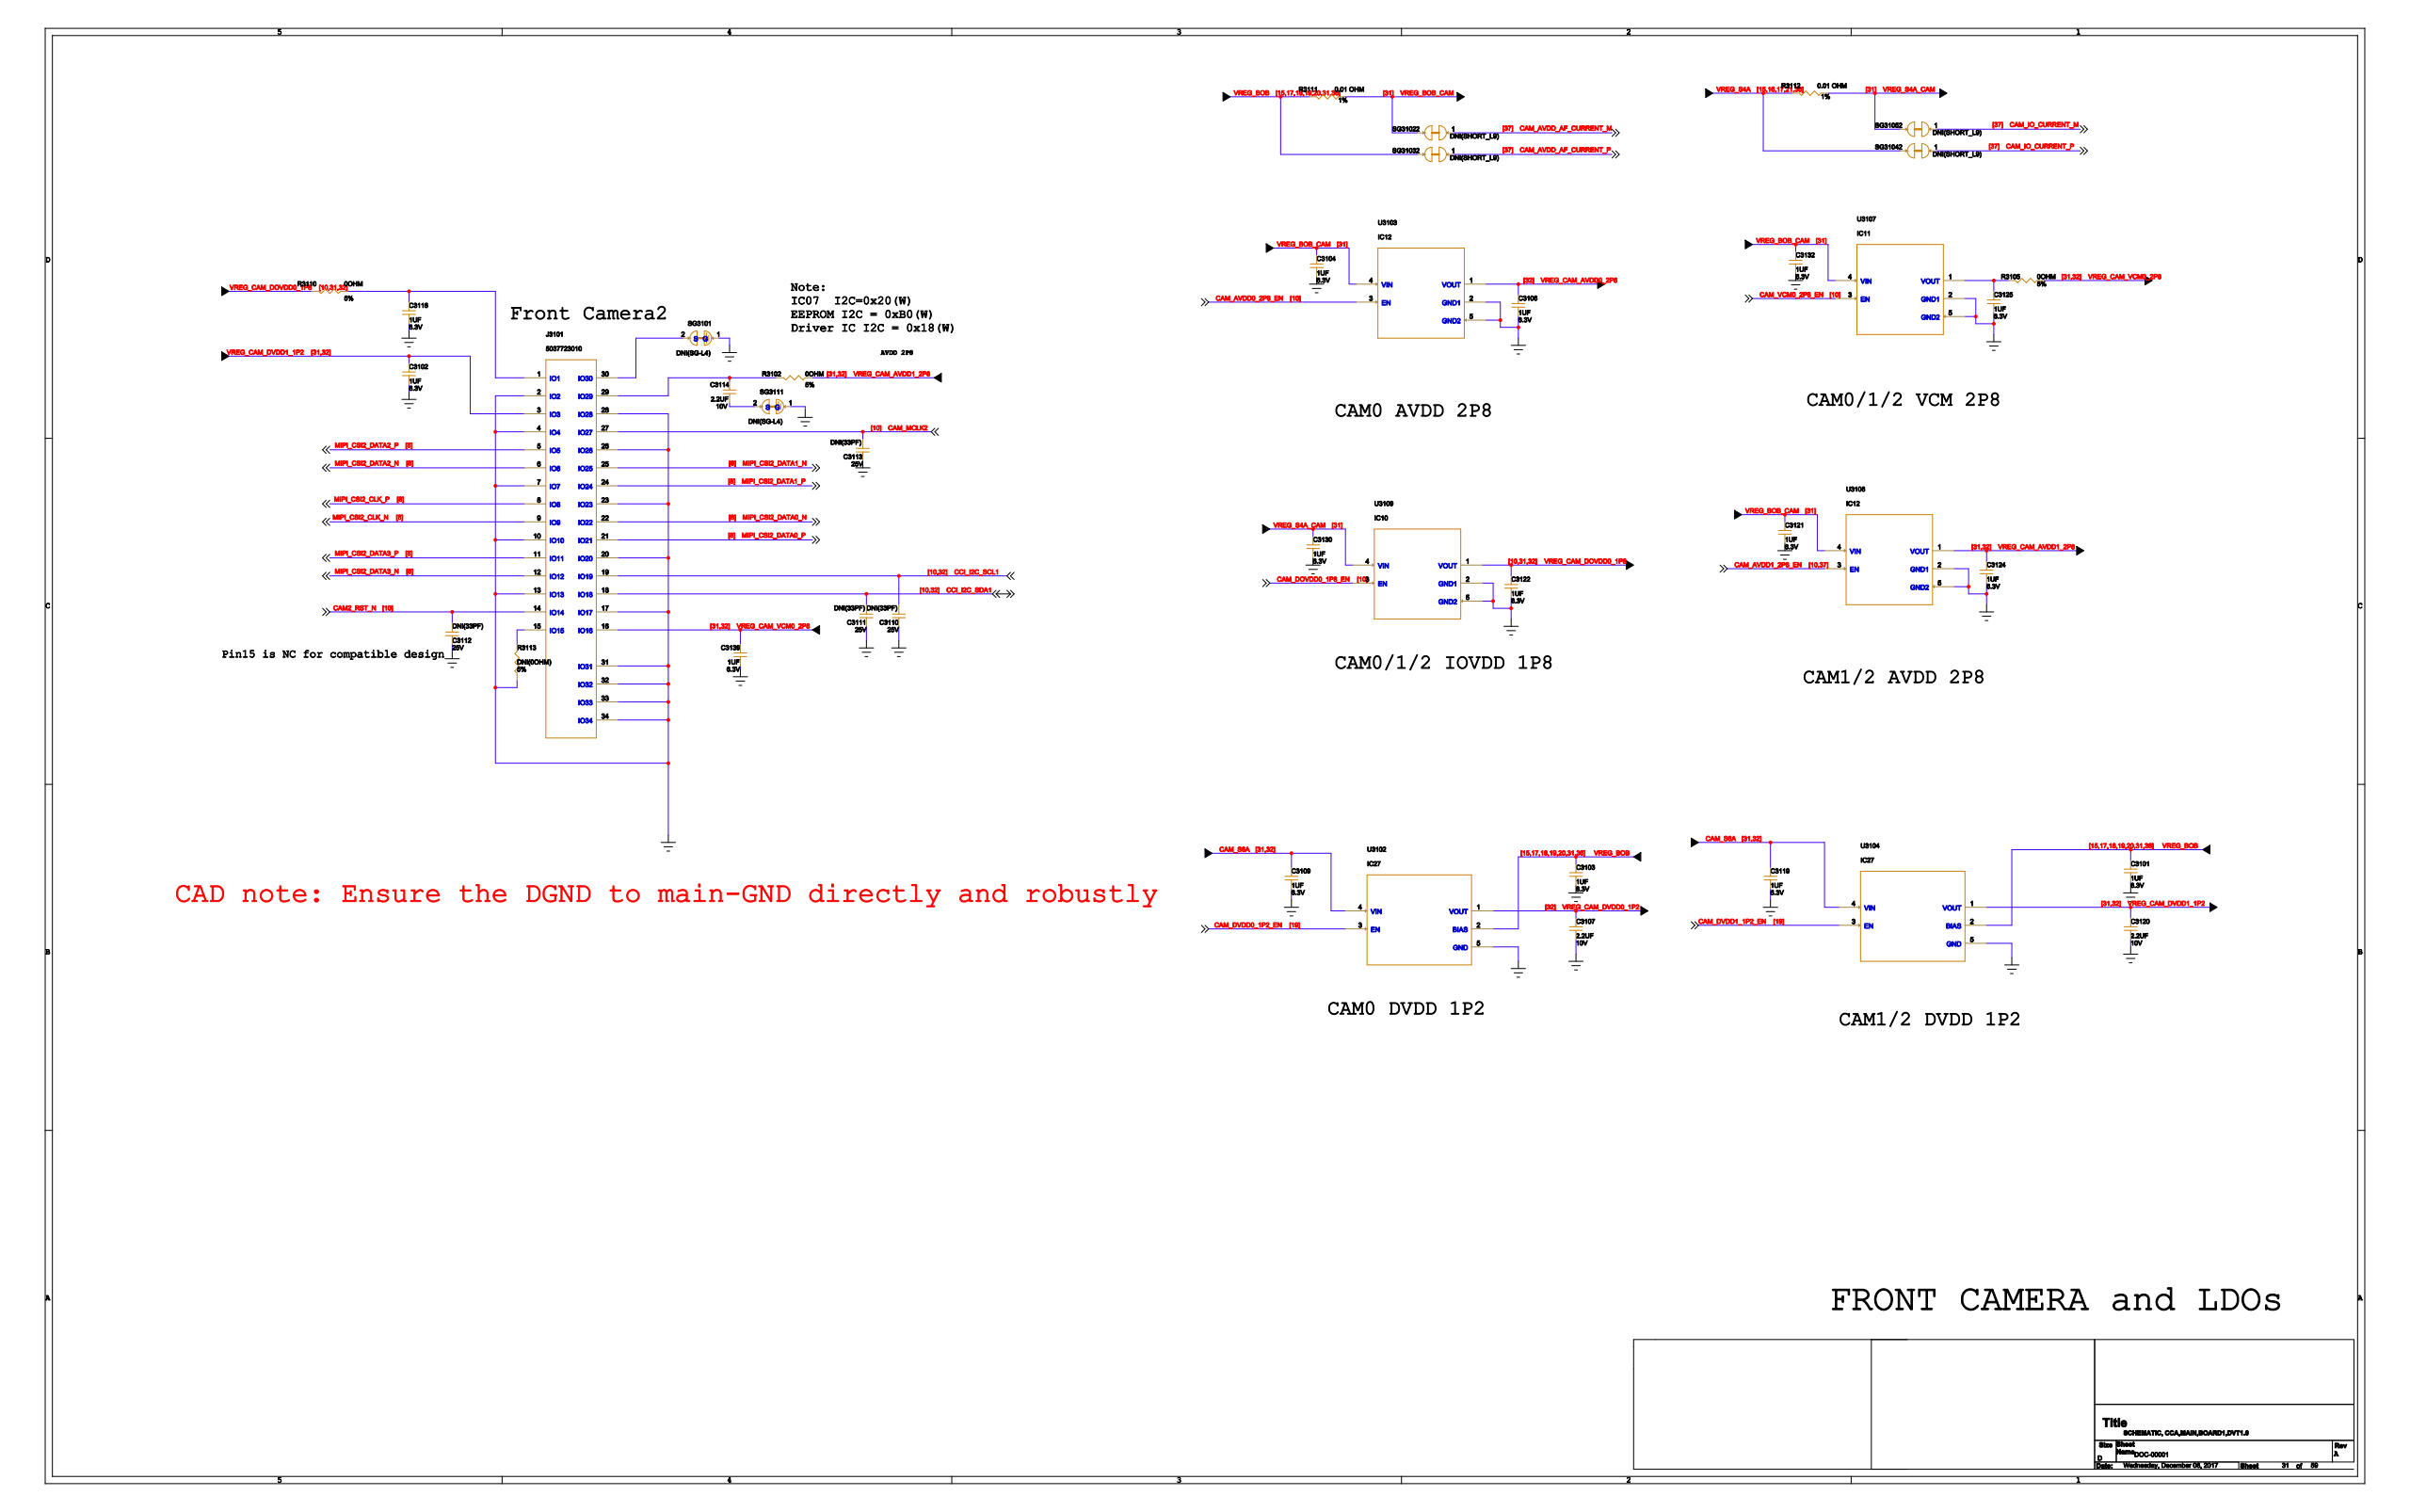Circuit board | KiCad | 1657 parts | 1365 nets | one sheet of the schematic
Parts on this sheet (reference | value | footprint):
C3101
C3102
C3103
C3104
C3106
C3107
C3109
C3110
C3111
C3112
C3113
C3114
C3116
C3119
C3120
C3121
C3122
C3124
C3125
C3130
C3132
C3139
J3101
R3102
R3105
R3110
R3111
R3112
R3113
SG3101
SG3102
SG3103
SG3104
SG3105
SG3111
U3102
U3103
U3104
U3106
U3107
U3109
Nets of these parts (net: part-pin ...):
GND: C3101-2 C3102-2 C3103-2 C3104-2 C3106-2 C3107-2 C3109-2 C3110-1 C3111-1 C3112-1 C3113-1 C3116-2 C3119-2 C3120-2 C3121-2 C3122-2 C3124-2 C3125-2 C3130-2 C3132-2 C3139-2 R3113-2 SG3101-1 SG3111-1 U3102-5 U3103-2 U3103-5 U3104-5 U3106-2 U3106-5 U3107-2 U3107-5 U3109-2 U3109-5 J3101-2 J3101-4 J3101-7 J3101-10 J3101-13 J3101-17 J3101-20 J3101-23 J3101-26 J3101-28 J3101-31 J3101-32 J3101-33 J3101-34
N24154747: R3113-1 J3101-15
_CAM_DVDD1_1P2: C3102-1 C3120-1 U3104-1 J3101-3
_CAM_AVDD0_2P8: C3106-1 U3103-1
VREG_BOB: C3101-1 C3103-1 R3111-1 SG3103-2 U3102-2 U3104-2
CAM_DOVDD0_1P8: C3122-1 R3110-1 U3109-1
_CAM_AVDD1_2P8: C3124-1 R3102-1 U3106-1
N21599140: C3114-1 R3102-2 J3101-29
D_AF_CURRENT_P: SG3103-1
N21642118: C3125-1 R3105-1 U3107-1
CAM_MCLK2: C3113-2 J3101-27
N21599656: SG3101-2 J3101-30
CCI_I2C_SDA1: C3111-2 J3101-18
M_DVDD1_1P2_EN: U3104-3
CAM_S6A: C3109-1 C3119-1 U3102-4 U3104-4
VREG_BOB_CAM: C3104-1 C3121-1 C3132-1 R3111-2 SG3102-2 U3103-4 U3106-4 U3107-4
AM_VCM0_2P8_EN: U3107-3
M_IO_CURRENT_M: SG3105-1
VREG_S4A_CAM: C3130-1 R3112-2 SG3105-2 U3109-4
N21599026: C3114-2 SG3111-2
CCI_I2C_SCL1: C3110-2 J3101-19
M_AVDD1_2P8_EN: U3106-3
M_AVDD0_2P8_EN: U3103-3
M_IO_CURRENT_P: SG3104-1
VREG_S4A: R3112-1 SG3104-2
_CAM_DVDD0_1P2: C3107-1 U3102-1
G_CAM_VCM0_2P8: C3139-1 R3105-2 J3101-16
M_DVDD0_1P2_EN: U3102-3
D_AF_CURRENT_M: SG3102-1
_DOVDD0_1P8_EN: U3109-3
CAM2_RST_N: C3112-2 J3101-14
N21590138: C3116-1 R3110-2 J3101-1